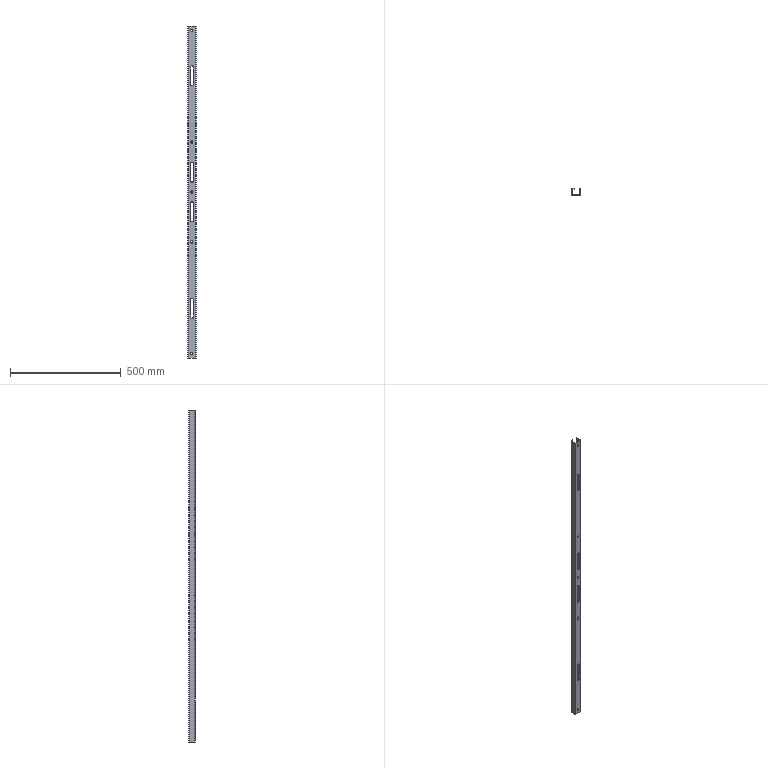Part | SolidWorks | features FlatPattern 1, ICE 1, SMBaseFlange 1, SheetMetal 1 | 1 solid | 75 faces | box 37 x 30 x 1500 mm | volume 289568 mm3 | plane 42 | cylinder 33 | commonest cylinder face diameters 9 x15 11 x12 2 x3 6 x3